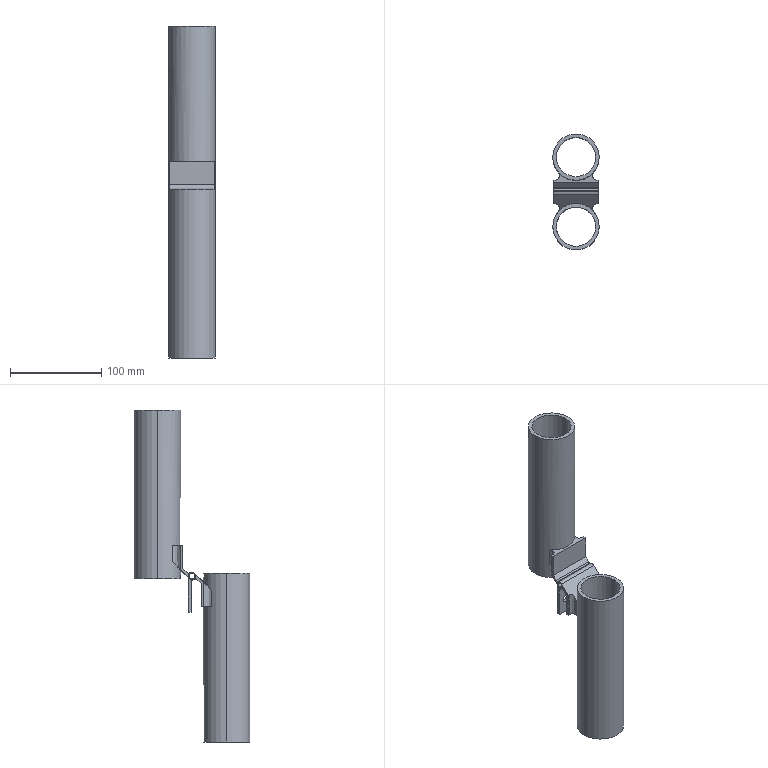Part | CATIA | 2 solids | 51 faces | box 51 x 127 x 364.6 mm | volume 241674 mm3 | cylinder 24 | plane 23 | spline 4 | commonest cylinder face diameters 6 x5 5.766 x4 8.5 x4 43 x4 51 x4 8 x3